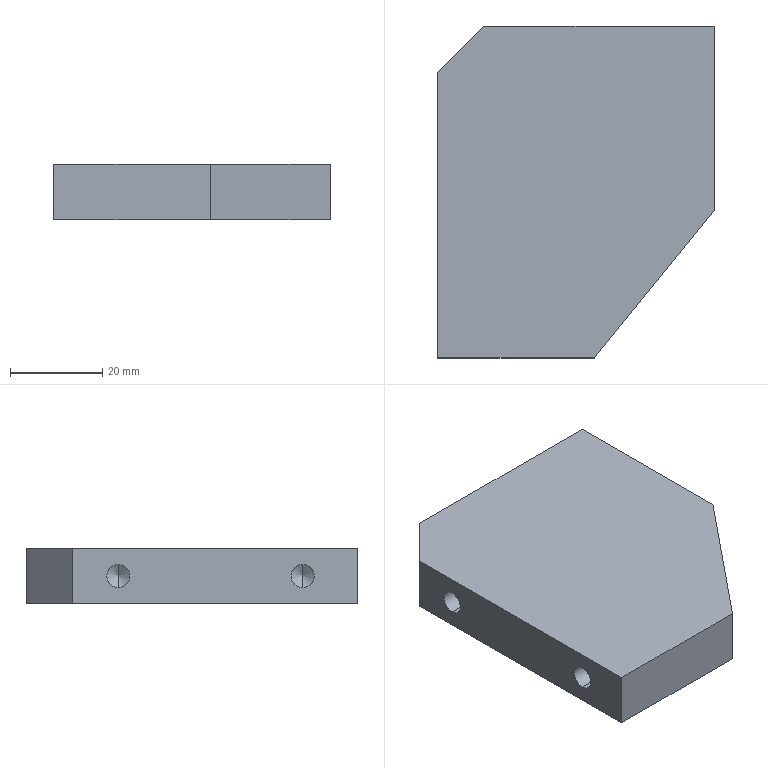Part | SolidWorks | features HoleWzd 2, Chamfer 1, Extrusion 1 | 1 solid | 24 faces | box 60 x 72 x 12 mm | volume 45188 mm3 | cylinder 8 | cone 8 | plane 8 | commonest cylinder face diameters 5 x8
STEP:
#1=CARTESIAN_POINT('',(-86.999,-8.,3.5));
#2=VERTEX_POINT('',#1);
#3=CARTESIAN_POINT('',(-86.999,-8.,8.5));
#4=VERTEX_POINT('',#3);
#5=CARTESIAN_POINT('',(-86.999,-8.,6.));
#6=DIRECTION('',(-1.,0.,0.));
#7=DIRECTION('',(0.,0.,1.));
#8=AXIS2_PLACEMENT_3D('',#5,#6,#7);
#9=CIRCLE('',#8,2.5);
#10=EDGE_CURVE('',#2,#4,#9,.T.);
#11=ORIENTED_EDGE('',*,*,#10,.F.);
#12=CARTESIAN_POINT('',(-99.999,-8.,3.5));
#13=VERTEX_POINT('',#12);
#14=CARTESIAN_POINT('',(-99.999,-8.,3.5));
#15=DIRECTION('',(-1.,0.,0.));
#16=VECTOR('',#15,1000.);
#17=LINE('',#14,#16);
#18=EDGE_CURVE('',#2,#13,#17,.T.);
#19=ORIENTED_EDGE('',*,*,#18,.T.);
#20=CARTESIAN_POINT('',(-99.999,-8.,8.5));
#21=VERTEX_POINT('',#20);
#22=CARTESIAN_POINT('',(-99.999,-8.,6.));
#23=DIRECTION('',(-1.,0.,0.));
#24=DIRECTION('',(0.,0.,1.));
#25=AXIS2_PLACEMENT_3D('',#22,#23,#24);
#26=CIRCLE('',#25,2.5);
#27=EDGE_CURVE('',#13,#21,#26,.T.);
#28=ORIENTED_EDGE('',*,*,#27,.T.);
#29=CARTESIAN_POINT('',(-99.999,-8.,8.5));
#30=DIRECTION('',(-1.,0.,0.));
#31=VECTOR('',#30,1000.);
#32=LINE('',#29,#31);
#33=EDGE_CURVE('',#4,#21,#32,.T.);
#34=ORIENTED_EDGE('',*,*,#33,.F.);
#35=EDGE_LOOP('',(#11,#19,#28,#34));
#36=FACE_OUTER_BOUND('',#35,.T.);
#37=CARTESIAN_POINT('',(-99.999,-8.,6.));
#38=DIRECTION('',(-1.,0.,0.));
#39=DIRECTION('',(0.,0.,1.));
#40=AXIS2_PLACEMENT_3D('',#37,#38,#39);
#41=CYLINDRICAL_SURFACE('',#40,2.5);
#42=ADVANCED_FACE('',(#36),#41,.F.);
#43=CARTESIAN_POINT('',(-85.496,-8.,6.));
#44=VERTEX_POINT('',#43);
#45=CARTESIAN_POINT('',(-86.999,-8.,8.5));
#46=DIRECTION('',(-0.515,0.,0.8572));
#47=VECTOR('',#46,1000.);
#48=LINE('',#45,#47);
#49=EDGE_CURVE('',#44,#4,#48,.T.);
#50=ORIENTED_EDGE('',*,*,#49,.F.);
#51=CARTESIAN_POINT('',(-86.999,-8.,3.5));
#52=DIRECTION('',(-0.515,0.,-0.8572));
#53=VECTOR('',#52,1000.);
#54=LINE('',#51,#53);
#55=EDGE_CURVE('',#44,#2,#54,.T.);
#56=ORIENTED_EDGE('',*,*,#55,.T.);
#57=ORIENTED_EDGE('',*,*,#10,.T.);
#58=EDGE_LOOP('',(#50,#56,#57));
#59=FACE_OUTER_BOUND('',#58,.T.);
#60=CARTESIAN_POINT('',(-86.999,-8.,6.));
#61=DIRECTION('',(-1.,0.,0.));
#62=DIRECTION('',(0.,0.,1.));
#63=AXIS2_PLACEMENT_3D('',#60,#61,#62);
#64=CONICAL_SURFACE('',#63,2.5,1.03);
#65=ADVANCED_FACE('',(#59),#64,.F.);
#66=CARTESIAN_POINT('',(-86.999,-48.,3.5));
#67=VERTEX_POINT('',#66);
#68=CARTESIAN_POINT('',(-86.999,-48.,8.5));
#69=VERTEX_POINT('',#68);
#70=CARTESIAN_POINT('',(-86.999,-48.,6.));
#71=DIRECTION('',(-1.,0.,0.));
#72=DIRECTION('',(0.,0.,1.));
#73=AXIS2_PLACEMENT_3D('',#70,#71,#72);
#74=CIRCLE('',#73,2.5);
#75=EDGE_CURVE('',#67,#69,#74,.T.);
#76=ORIENTED_EDGE('',*,*,#75,.F.);
#77=CARTESIAN_POINT('',(-99.999,-48.,3.5));
#78=VERTEX_POINT('',#77);
#79=CARTESIAN_POINT('',(-99.999,-48.,3.5));
#80=DIRECTION('',(-1.,0.,0.));
#81=VECTOR('',#80,1000.);
#82=LINE('',#79,#81);
#83=EDGE_CURVE('',#67,#78,#82,.T.);
#84=ORIENTED_EDGE('',*,*,#83,.T.);
#85=CARTESIAN_POINT('',(-99.999,-48.,8.5));
#86=VERTEX_POINT('',#85);
#87=CARTESIAN_POINT('',(-99.999,-48.,6.));
#88=DIRECTION('',(-1.,0.,0.));
#89=DIRECTION('',(0.,0.,1.));
#90=AXIS2_PLACEMENT_3D('',#87,#88,#89);
#91=CIRCLE('',#90,2.5);
#92=EDGE_CURVE('',#78,#86,#91,.T.);
#93=ORIENTED_EDGE('',*,*,#92,.T.);
#94=CARTESIAN_POINT('',(-99.999,-48.,8.5));
#95=DIRECTION('',(-1.,0.,0.));
#96=VECTOR('',#95,1000.);
#97=LINE('',#94,#96);
#98=EDGE_CURVE('',#69,#86,#97,.T.);
#99=ORIENTED_EDGE('',*,*,#98,.F.);
#100=EDGE_LOOP('',(#76,#84,#93,#99));
#101=FACE_OUTER_BOUND('',#100,.T.);
#102=CARTESIAN_POINT('',(-99.999,-48.,6.));
#103=DIRECTION('',(-1.,0.,0.));
#104=DIRECTION('',(0.,0.,1.));
#105=AXIS2_PLACEMENT_3D('',#102,#103,#104);
#106=CYLINDRICAL_SURFACE('',#105,2.5);
#107=ADVANCED_FACE('',(#101),#106,.F.);
#108=CARTESIAN_POINT('',(-85.496,-48.,6.));
#109=VERTEX_POINT('',#108);
#110=CARTESIAN_POINT('',(-86.999,-48.,8.5));
#111=DIRECTION('',(-0.515,0.,0.8572));
#112=VECTOR('',#111,1000.);
#113=LINE('',#110,#112);
#114=EDGE_CURVE('',#109,#69,#113,.T.);
#115=ORIENTED_EDGE('',*,*,#114,.F.);
#116=CARTESIAN_POINT('',(-86.999,-48.,3.5));
#117=DIRECTION('',(-0.515,0.,-0.8572));
#118=VECTOR('',#117,1000.);
#119=LINE('',#116,#118);
#120=EDGE_CURVE('',#109,#67,#119,.T.);
#121=ORIENTED_EDGE('',*,*,#120,.T.);
#122=ORIENTED_EDGE('',*,*,#75,.T.);
#123=EDGE_LOOP('',(#115,#121,#122));
#124=FACE_OUTER_BOUND('',#123,.T.);
#125=CARTESIAN_POINT('',(-86.999,-48.,6.));
#126=DIRECTION('',(-1.,0.,0.));
#127=DIRECTION('',(0.,0.,1.));
#128=AXIS2_PLACEMENT_3D('',#125,#126,#127);
#129=CONICAL_SURFACE('',#128,2.5,1.03);
#130=ADVANCED_FACE('',(#124),#129,.F.);
#131=CARTESIAN_POINT('',(-52.999,4.,8.5));
#132=VERTEX_POINT('',#131);
#133=CARTESIAN_POINT('',(-52.999,4.,3.5));
#134=VERTEX_POINT('',#133);
#135=CARTESIAN_POINT('',(-52.999,4.,6.));
#136=DIRECTION('',(1.,0.,0.));
#137=DIRECTION('',(0.,0.,-1.));
#138=AXIS2_PLACEMENT_3D('',#135,#136,#137);
#139=CIRCLE('',#138,2.5);
#140=EDGE_CURVE('',#132,#134,#139,.T.);
#141=ORIENTED_EDGE('',*,*,#140,.F.);
#142=CARTESIAN_POINT('',(-39.999,4.,8.5));
#143=VERTEX_POINT('',#142);
#144=CARTESIAN_POINT('',(-39.999,4.,8.5));
#145=DIRECTION('',(1.,0.,0.));
#146=VECTOR('',#145,1000.);
#147=LINE('',#144,#146);
#148=EDGE_CURVE('',#132,#143,#147,.T.);
#149=ORIENTED_EDGE('',*,*,#148,.T.);
#150=CARTESIAN_POINT('',(-39.999,4.,3.5));
#151=VERTEX_POINT('',#150);
#152=CARTESIAN_POINT('',(-39.999,4.,6.));
#153=DIRECTION('',(1.,0.,0.));
#154=DIRECTION('',(0.,0.,-1.));
#155=AXIS2_PLACEMENT_3D('',#152,#153,#154);
#156=CIRCLE('',#155,2.5);
#157=EDGE_CURVE('',#143,#151,#156,.T.);
#158=ORIENTED_EDGE('',*,*,#157,.T.);
#159=CARTESIAN_POINT('',(-39.999,4.,3.5));
#160=DIRECTION('',(1.,0.,0.));
#161=VECTOR('',#160,1000.);
#162=LINE('',#159,#161);
#163=EDGE_CURVE('',#134,#151,#162,.T.);
#164=ORIENTED_EDGE('',*,*,#163,.F.);
#165=EDGE_LOOP('',(#141,#149,#158,#164));
#166=FACE_OUTER_BOUND('',#165,.T.);
#167=CARTESIAN_POINT('',(-39.999,4.,6.));
#168=DIRECTION('',(1.,0.,0.));
#169=DIRECTION('',(0.,0.,-1.));
#170=AXIS2_PLACEMENT_3D('',#167,#168,#169);
#171=CYLINDRICAL_SURFACE('',#170,2.5);
#172=ADVANCED_FACE('',(#166),#171,.F.);
#173=CARTESIAN_POINT('',(-54.501,4.,6.));
#174=VERTEX_POINT('',#173);
#175=CARTESIAN_POINT('',(-52.999,4.,3.5));
#176=DIRECTION('',(0.515,0.,-0.8572));
#177=VECTOR('',#176,1000.);
#178=LINE('',#175,#177);
#179=EDGE_CURVE('',#174,#134,#178,.T.);
#180=ORIENTED_EDGE('',*,*,#179,.F.);
#181=CARTESIAN_POINT('',(-52.999,4.,8.5));
#182=DIRECTION('',(0.515,0.,0.8572));
#183=VECTOR('',#182,1000.);
#184=LINE('',#181,#183);
#185=EDGE_CURVE('',#174,#132,#184,.T.);
#186=ORIENTED_EDGE('',*,*,#185,.T.);
#187=ORIENTED_EDGE('',*,*,#140,.T.);
#188=EDGE_LOOP('',(#180,#186,#187));
#189=FACE_OUTER_BOUND('',#188,.T.);
#190=CARTESIAN_POINT('',(-52.999,4.,6.));
#191=DIRECTION('',(1.,0.,0.));
#192=DIRECTION('',(0.,0.,-1.));
#193=AXIS2_PLACEMENT_3D('',#190,#191,#192);
#194=CONICAL_SURFACE('',#193,2.5,1.03);
#195=ADVANCED_FACE('',(#189),#194,.F.);
#196=CARTESIAN_POINT('',(-52.999,-16.,8.5));
#197=VERTEX_POINT('',#196);
#198=CARTESIAN_POINT('',(-52.999,-16.,3.5));
#199=VERTEX_POINT('',#198);
#200=CARTESIAN_POINT('',(-52.999,-16.,6.));
#201=DIRECTION('',(1.,0.,0.));
#202=DIRECTION('',(0.,0.,-1.));
#203=AXIS2_PLACEMENT_3D('',#200,#201,#202);
#204=CIRCLE('',#203,2.5);
#205=EDGE_CURVE('',#197,#199,#204,.T.);
#206=ORIENTED_EDGE('',*,*,#205,.F.);
#207=CARTESIAN_POINT('',(-39.999,-16.,8.5));
#208=VERTEX_POINT('',#207);
#209=CARTESIAN_POINT('',(-39.999,-16.,8.5));
#210=DIRECTION('',(1.,0.,0.));
#211=VECTOR('',#210,1000.);
#212=LINE('',#209,#211);
#213=EDGE_CURVE('',#197,#208,#212,.T.);
#214=ORIENTED_EDGE('',*,*,#213,.T.);
#215=CARTESIAN_POINT('',(-39.999,-16.,3.5));
#216=VERTEX_POINT('',#215);
#217=CARTESIAN_POINT('',(-39.999,-16.,6.));
#218=DIRECTION('',(1.,0.,0.));
#219=DIRECTION('',(0.,0.,-1.));
#220=AXIS2_PLACEMENT_3D('',#217,#218,#219);
#221=CIRCLE('',#220,2.5);
#222=EDGE_CURVE('',#208,#216,#221,.T.);
#223=ORIENTED_EDGE('',*,*,#222,.T.);
#224=CARTESIAN_POINT('',(-39.999,-16.,3.5));
#225=DIRECTION('',(1.,0.,0.));
#226=VECTOR('',#225,1000.);
#227=LINE('',#224,#226);
#228=EDGE_CURVE('',#199,#216,#227,.T.);
#229=ORIENTED_EDGE('',*,*,#228,.F.);
#230=EDGE_LOOP('',(#206,#214,#223,#229));
#231=FACE_OUTER_BOUND('',#230,.T.);
#232=CARTESIAN_POINT('',(-39.999,-16.,6.));
#233=DIRECTION('',(1.,0.,0.));
#234=DIRECTION('',(0.,0.,-1.));
#235=AXIS2_PLACEMENT_3D('',#232,#233,#234);
#236=CYLINDRICAL_SURFACE('',#235,2.5);
#237=ADVANCED_FACE('',(#231),#236,.F.);
#238=CARTESIAN_POINT('',(-54.501,-16.,6.));
#239=VERTEX_POINT('',#238);
#240=CARTESIAN_POINT('',(-52.999,-16.,3.5));
#241=DIRECTION('',(0.515,0.,-0.8572));
#242=VECTOR('',#241,1000.);
#243=LINE('',#240,#242);
#244=EDGE_CURVE('',#239,#199,#243,.T.);
#245=ORIENTED_EDGE('',*,*,#244,.F.);
#246=CARTESIAN_POINT('',(-52.999,-16.,8.5));
#247=DIRECTION('',(0.515,0.,0.8572));
#248=VECTOR('',#247,1000.);
#249=LINE('',#246,#248);
#250=EDGE_CURVE('',#239,#197,#249,.T.);
#251=ORIENTED_EDGE('',*,*,#250,.T.);
#252=ORIENTED_EDGE('',*,*,#205,.T.);
#253=EDGE_LOOP('',(#245,#251,#252));
#254=FACE_OUTER_BOUND('',#253,.T.);
#255=CARTESIAN_POINT('',(-52.999,-16.,6.));
#256=DIRECTION('',(1.,0.,0.));
#257=DIRECTION('',(0.,0.,-1.));
#258=AXIS2_PLACEMENT_3D('',#255,#256,#257);
#259=CONICAL_SURFACE('',#258,2.5,1.03);
#260=ADVANCED_FACE('',(#254),#259,.F.);
#261=CARTESIAN_POINT('',(-39.999,12.,0.));
#262=VERTEX_POINT('',#261);
#263=CARTESIAN_POINT('',(-89.999,12.,0.));
#264=VERTEX_POINT('',#263);
#265=CARTESIAN_POINT('',(-99.999,12.,0.));
#266=DIRECTION('',(-1.,0.,0.));
#267=VECTOR('',#266,1000.);
#268=LINE('',#265,#267);
#269=EDGE_CURVE('',#262,#264,#268,.T.);
#270=ORIENTED_EDGE('',*,*,#269,.T.);
#271=CARTESIAN_POINT('',(-89.999,12.,12.));
#272=VERTEX_POINT('',#271);
#273=CARTESIAN_POINT('',(-89.999,12.,12.));
#274=DIRECTION('',(0.,0.,1.));
#275=VECTOR('',#274,1000.);
#276=LINE('',#273,#275);
#277=EDGE_CURVE('',#264,#272,#276,.T.);
#278=ORIENTED_EDGE('',*,*,#277,.T.);
#279=CARTESIAN_POINT('',(-39.999,12.,12.));
#280=VERTEX_POINT('',#279);
#281=CARTESIAN_POINT('',(-99.999,12.,12.));
#282=DIRECTION('',(-1.,0.,0.));
#283=VECTOR('',#282,1000.);
#284=LINE('',#281,#283);
#285=EDGE_CURVE('',#280,#272,#284,.T.);
#286=ORIENTED_EDGE('',*,*,#285,.F.);
#287=CARTESIAN_POINT('',(-39.999,12.,12.));
#288=DIRECTION('',(0.,0.,-1.));
#289=VECTOR('',#288,1000.);
#290=LINE('',#287,#289);
#291=EDGE_CURVE('',#280,#262,#290,.T.);
#292=ORIENTED_EDGE('',*,*,#291,.T.);
#293=EDGE_LOOP('',(#270,#278,#286,#292));
#294=FACE_OUTER_BOUND('',#293,.T.);
#295=CARTESIAN_POINT('',(-99.999,12.,12.));
#296=DIRECTION('',(0.,-1.,0.));
#297=DIRECTION('',(1.,0.,0.));
#298=AXIS2_PLACEMENT_3D('',#295,#296,#297);
#299=PLANE('',#298);
#300=ADVANCED_FACE('',(#294),#299,.F.);
#301=CARTESIAN_POINT('',(-99.999,-8.,6.));
#302=DIRECTION('',(-1.,0.,0.));
#303=DIRECTION('',(0.,0.,1.));
#304=AXIS2_PLACEMENT_3D('',#301,#302,#303);
#305=CIRCLE('',#304,2.5);
#306=EDGE_CURVE('',#21,#13,#305,.T.);
#307=ORIENTED_EDGE('',*,*,#306,.F.);
#308=ORIENTED_EDGE('',*,*,#27,.F.);
#309=EDGE_LOOP('',(#307,#308));
#310=FACE_BOUND('',#309,.T.);
#311=CARTESIAN_POINT('',(-99.999,-48.,6.));
#312=DIRECTION('',(-1.,0.,0.));
#313=DIRECTION('',(0.,0.,1.));
#314=AXIS2_PLACEMENT_3D('',#311,#312,#313);
#315=CIRCLE('',#314,2.5);
#316=EDGE_CURVE('',#86,#78,#315,.T.);
#317=ORIENTED_EDGE('',*,*,#316,.F.);
#318=ORIENTED_EDGE('',*,*,#92,.F.);
#319=EDGE_LOOP('',(#317,#318));
#320=FACE_BOUND('',#319,.T.);
#321=CARTESIAN_POINT('',(-99.999,2.,12.));
#322=VERTEX_POINT('',#321);
#323=CARTESIAN_POINT('',(-99.999,-60.,12.));
#324=VERTEX_POINT('',#323);
#325=CARTESIAN_POINT('',(-99.999,-60.,12.));
#326=DIRECTION('',(0.,-1.,0.));
#327=VECTOR('',#326,1000.);
#328=LINE('',#325,#327);
#329=EDGE_CURVE('',#322,#324,#328,.T.);
#330=ORIENTED_EDGE('',*,*,#329,.F.);
#331=CARTESIAN_POINT('',(-99.999,2.,0.));
#332=VERTEX_POINT('',#331);
#333=CARTESIAN_POINT('',(-99.999,2.,12.));
#334=DIRECTION('',(0.,0.,-1.));
#335=VECTOR('',#334,1000.);
#336=LINE('',#333,#335);
#337=EDGE_CURVE('',#322,#332,#336,.T.);
#338=ORIENTED_EDGE('',*,*,#337,.T.);
#339=CARTESIAN_POINT('',(-99.999,-60.,0.));
#340=VERTEX_POINT('',#339);
#341=CARTESIAN_POINT('',(-99.999,-60.,0.));
#342=DIRECTION('',(0.,-1.,0.));
#343=VECTOR('',#342,1000.);
#344=LINE('',#341,#343);
#345=EDGE_CURVE('',#332,#340,#344,.T.);
#346=ORIENTED_EDGE('',*,*,#345,.T.);
#347=CARTESIAN_POINT('',(-99.999,-60.,12.));
#348=DIRECTION('',(0.,0.,-1.));
#349=VECTOR('',#348,1000.);
#350=LINE('',#347,#349);
#351=EDGE_CURVE('',#324,#340,#350,.T.);
#352=ORIENTED_EDGE('',*,*,#351,.F.);
#353=EDGE_LOOP('',(#330,#338,#346,#352));
#354=FACE_OUTER_BOUND('',#353,.T.);
#355=CARTESIAN_POINT('',(-99.999,-60.,12.));
#356=DIRECTION('',(1.,0.,0.));
#357=DIRECTION('',(0.,0.,-1.));
#358=AXIS2_PLACEMENT_3D('',#355,#356,#357);
#359=PLANE('',#358);
#360=ADVANCED_FACE('',(#310,#320,#354),#359,.F.);
#361=CARTESIAN_POINT('',(-65.999,-60.,0.));
#362=VERTEX_POINT('',#361);
#363=CARTESIAN_POINT('',(-99.999,-60.,0.));
#364=DIRECTION('',(1.,0.,0.));
#365=VECTOR('',#364,1000.);
#366=LINE('',#363,#365);
#367=EDGE_CURVE('',#340,#362,#366,.T.);
#368=ORIENTED_EDGE('',*,*,#367,.T.);
#369=CARTESIAN_POINT('',(-65.999,-60.,12.));
#370=VERTEX_POINT('',#369);
#371=CARTESIAN_POINT('',(-65.999,-60.,12.));
#372=DIRECTION('',(0.,0.,-1.));
#373=VECTOR('',#372,1000.);
#374=LINE('',#371,#373);
#375=EDGE_CURVE('',#370,#362,#374,.T.);
#376=ORIENTED_EDGE('',*,*,#375,.F.);
#377=CARTESIAN_POINT('',(-99.999,-60.,12.));
#378=DIRECTION('',(1.,0.,0.));
#379=VECTOR('',#378,1000.);
#380=LINE('',#377,#379);
#381=EDGE_CURVE('',#324,#370,#380,.T.);
#382=ORIENTED_EDGE('',*,*,#381,.F.);
#383=ORIENTED_EDGE('',*,*,#351,.T.);
#384=EDGE_LOOP('',(#368,#376,#382,#383));
#385=FACE_OUTER_BOUND('',#384,.T.);
#386=CARTESIAN_POINT('',(-99.999,-60.,12.));
#387=DIRECTION('',(0.,1.,0.));
#388=DIRECTION('',(-1.,0.,0.));
#389=AXIS2_PLACEMENT_3D('',#386,#387,#388);
#390=PLANE('',#389);
#391=ADVANCED_FACE('',(#385),#390,.F.);
#392=CARTESIAN_POINT('',(-39.999,-28.,0.));
#393=VERTEX_POINT('',#392);
#394=CARTESIAN_POINT('',(-65.999,-60.,0.));
#395=DIRECTION('',(0.6306,0.7761,0.));
#396=VECTOR('',#395,1000.);
#397=LINE('',#394,#396);
#398=EDGE_CURVE('',#362,#393,#397,.T.);
#399=ORIENTED_EDGE('',*,*,#398,.T.);
#400=CARTESIAN_POINT('',(-39.999,-28.,12.));
#401=VERTEX_POINT('',#400);
#402=CARTESIAN_POINT('',(-39.999,-28.,12.));
#403=DIRECTION('',(0.,0.,-1.));
#404=VECTOR('',#403,1000.);
#405=LINE('',#402,#404);
#406=EDGE_CURVE('',#401,#393,#405,.T.);
#407=ORIENTED_EDGE('',*,*,#406,.F.);
#408=CARTESIAN_POINT('',(-65.999,-60.,12.));
#409=DIRECTION('',(0.6306,0.7761,0.));
#410=VECTOR('',#409,1000.);
#411=LINE('',#408,#410);
#412=EDGE_CURVE('',#370,#401,#411,.T.);
#413=ORIENTED_EDGE('',*,*,#412,.F.);
#414=ORIENTED_EDGE('',*,*,#375,.T.);
#415=EDGE_LOOP('',(#399,#407,#413,#414));
#416=FACE_OUTER_BOUND('',#415,.T.);
#417=CARTESIAN_POINT('',(-65.999,-60.,12.));
#418=DIRECTION('',(-0.7761,0.6306,0.));
#419=DIRECTION('',(-0.6306,-0.7761,0.));
#420=AXIS2_PLACEMENT_3D('',#417,#418,#419);
#421=PLANE('',#420);
#422=ADVANCED_FACE('',(#416),#421,.F.);
#423=CARTESIAN_POINT('',(-39.999,4.,6.));
#424=DIRECTION('',(1.,0.,0.));
#425=DIRECTION('',(0.,0.,-1.));
#426=AXIS2_PLACEMENT_3D('',#423,#424,#425);
#427=CIRCLE('',#426,2.5);
#428=EDGE_CURVE('',#151,#143,#427,.T.);
#429=ORIENTED_EDGE('',*,*,#428,.F.);
#430=ORIENTED_EDGE('',*,*,#157,.F.);
#431=EDGE_LOOP('',(#429,#430));
#432=FACE_BOUND('',#431,.T.);
#433=CARTESIAN_POINT('',(-39.999,-16.,6.));
#434=DIRECTION('',(1.,0.,0.));
#435=DIRECTION('',(0.,0.,-1.));
#436=AXIS2_PLACEMENT_3D('',#433,#434,#435);
#437=CIRCLE('',#436,2.5);
#438=EDGE_CURVE('',#216,#208,#437,.T.);
#439=ORIENTED_EDGE('',*,*,#438,.F.);
#440=ORIENTED_EDGE('',*,*,#222,.F.);
#441=EDGE_LOOP('',(#439,#440));
#442=FACE_BOUND('',#441,.T.);
#443=CARTESIAN_POINT('',(-39.999,12.,0.));
#444=DIRECTION('',(0.,1.,0.));
#445=VECTOR('',#444,1000.);
#446=LINE('',#443,#445);
#447=EDGE_CURVE('',#393,#262,#446,.T.);
#448=ORIENTED_EDGE('',*,*,#447,.T.);
#449=ORIENTED_EDGE('',*,*,#291,.F.);
#450=CARTESIAN_POINT('',(-39.999,12.,12.));
#451=DIRECTION('',(0.,1.,0.));
#452=VECTOR('',#451,1000.);
#453=LINE('',#450,#452);
#454=EDGE_CURVE('',#401,#280,#453,.T.);
#455=ORIENTED_EDGE('',*,*,#454,.F.);
#456=ORIENTED_EDGE('',*,*,#406,.T.);
#457=EDGE_LOOP('',(#448,#449,#455,#456));
#458=FACE_OUTER_BOUND('',#457,.T.);
#459=CARTESIAN_POINT('',(-39.999,12.,12.));
#460=DIRECTION('',(-1.,0.,0.));
#461=DIRECTION('',(0.,-1.,0.));
#462=AXIS2_PLACEMENT_3D('',#459,#460,#461);
#463=PLANE('',#462);
#464=ADVANCED_FACE('',(#432,#442,#458),#463,.F.);
#465=ORIENTED_EDGE('',*,*,#285,.T.);
#466=CARTESIAN_POINT('',(-99.999,2.,12.));
#467=DIRECTION('',(-0.7071,-0.7071,0.));
#468=VECTOR('',#467,1000.);
#469=LINE('',#466,#468);
#470=EDGE_CURVE('',#272,#322,#469,.T.);
#471=ORIENTED_EDGE('',*,*,#470,.T.);
#472=ORIENTED_EDGE('',*,*,#329,.T.);
#473=ORIENTED_EDGE('',*,*,#381,.T.);
#474=ORIENTED_EDGE('',*,*,#412,.T.);
#475=ORIENTED_EDGE('',*,*,#454,.T.);
#476=EDGE_LOOP('',(#465,#471,#472,#473,#474,#475));
#477=FACE_OUTER_BOUND('',#476,.T.);
#478=CARTESIAN_POINT('',(0.,0.,12.));
#479=DIRECTION('',(0.,0.,-1.));
#480=DIRECTION('',(-1.,0.,0.));
#481=AXIS2_PLACEMENT_3D('',#478,#479,#480);
#482=PLANE('',#481);
#483=ADVANCED_FACE('',(#477),#482,.F.);
#484=ORIENTED_EDGE('',*,*,#345,.F.);
#485=CARTESIAN_POINT('',(-50.999,50.999,0.));
#486=DIRECTION('',(0.7071,0.7071,0.));
#487=VECTOR('',#486,1000.);
#488=LINE('',#485,#487);
#489=EDGE_CURVE('',#332,#264,#488,.T.);
#490=ORIENTED_EDGE('',*,*,#489,.T.);
#491=ORIENTED_EDGE('',*,*,#269,.F.);
#492=ORIENTED_EDGE('',*,*,#447,.F.);
#493=ORIENTED_EDGE('',*,*,#398,.F.);
#494=ORIENTED_EDGE('',*,*,#367,.F.);
#495=EDGE_LOOP('',(#484,#490,#491,#492,#493,#494));
#496=FACE_OUTER_BOUND('',#495,.T.);
#497=CARTESIAN_POINT('',(0.,0.,0.));
#498=DIRECTION('',(0.,0.,-1.));
#499=DIRECTION('',(-1.,0.,0.));
#500=AXIS2_PLACEMENT_3D('',#497,#498,#499);
#501=PLANE('',#500);
#502=ADVANCED_FACE('',(#496),#501,.T.);
#503=ORIENTED_EDGE('',*,*,#470,.F.);
#504=ORIENTED_EDGE('',*,*,#277,.F.);
#505=ORIENTED_EDGE('',*,*,#489,.F.);
#506=ORIENTED_EDGE('',*,*,#337,.F.);
#507=EDGE_LOOP('',(#503,#504,#505,#506));
#508=FACE_OUTER_BOUND('',#507,.T.);
#509=CARTESIAN_POINT('',(-99.999,2.,12.));
#510=DIRECTION('',(0.7071,-0.7071,0.));
#511=DIRECTION('',(0.,0.,-1.));
#512=AXIS2_PLACEMENT_3D('',#509,#510,#511);
#513=PLANE('',#512);
#514=ADVANCED_FACE('',(#508),#513,.F.);
#515=ORIENTED_EDGE('',*,*,#250,.F.);
#516=ORIENTED_EDGE('',*,*,#244,.T.);
#517=CARTESIAN_POINT('',(-52.999,-16.,6.));
#518=DIRECTION('',(1.,0.,0.));
#519=DIRECTION('',(0.,0.,-1.));
#520=AXIS2_PLACEMENT_3D('',#517,#518,#519);
#521=CIRCLE('',#520,2.5);
#522=EDGE_CURVE('',#199,#197,#521,.T.);
#523=ORIENTED_EDGE('',*,*,#522,.T.);
#524=EDGE_LOOP('',(#515,#516,#523));
#525=FACE_OUTER_BOUND('',#524,.T.);
#526=CARTESIAN_POINT('',(-52.999,-16.,6.));
#527=DIRECTION('',(1.,0.,0.));
#528=DIRECTION('',(0.,0.,-1.));
#529=AXIS2_PLACEMENT_3D('',#526,#527,#528);
#530=CONICAL_SURFACE('',#529,2.5,1.03);
#531=ADVANCED_FACE('',(#525),#530,.F.);
#532=ORIENTED_EDGE('',*,*,#213,.F.);
#533=ORIENTED_EDGE('',*,*,#522,.F.);
#534=ORIENTED_EDGE('',*,*,#228,.T.);
#535=ORIENTED_EDGE('',*,*,#438,.T.);
#536=EDGE_LOOP('',(#532,#533,#534,#535));
#537=FACE_OUTER_BOUND('',#536,.T.);
#538=CARTESIAN_POINT('',(-39.999,-16.,6.));
#539=DIRECTION('',(1.,0.,0.));
#540=DIRECTION('',(0.,0.,-1.));
#541=AXIS2_PLACEMENT_3D('',#538,#539,#540);
#542=CYLINDRICAL_SURFACE('',#541,2.5);
#543=ADVANCED_FACE('',(#537),#542,.F.);
#544=ORIENTED_EDGE('',*,*,#185,.F.);
#545=ORIENTED_EDGE('',*,*,#179,.T.);
#546=CARTESIAN_POINT('',(-52.999,4.,6.));
#547=DIRECTION('',(1.,0.,0.));
#548=DIRECTION('',(0.,0.,-1.));
#549=AXIS2_PLACEMENT_3D('',#546,#547,#548);
#550=CIRCLE('',#549,2.5);
#551=EDGE_CURVE('',#134,#132,#550,.T.);
#552=ORIENTED_EDGE('',*,*,#551,.T.);
#553=EDGE_LOOP('',(#544,#545,#552));
#554=FACE_OUTER_BOUND('',#553,.T.);
#555=CARTESIAN_POINT('',(-52.999,4.,6.));
#556=DIRECTION('',(1.,0.,0.));
#557=DIRECTION('',(0.,0.,-1.));
#558=AXIS2_PLACEMENT_3D('',#555,#556,#557);
#559=CONICAL_SURFACE('',#558,2.5,1.03);
#560=ADVANCED_FACE('',(#554),#559,.F.);
#561=ORIENTED_EDGE('',*,*,#148,.F.);
#562=ORIENTED_EDGE('',*,*,#551,.F.);
#563=ORIENTED_EDGE('',*,*,#163,.T.);
#564=ORIENTED_EDGE('',*,*,#428,.T.);
#565=EDGE_LOOP('',(#561,#562,#563,#564));
#566=FACE_OUTER_BOUND('',#565,.T.);
#567=CARTESIAN_POINT('',(-39.999,4.,6.));
#568=DIRECTION('',(1.,0.,0.));
#569=DIRECTION('',(0.,0.,-1.));
#570=AXIS2_PLACEMENT_3D('',#567,#568,#569);
#571=CYLINDRICAL_SURFACE('',#570,2.5);
#572=ADVANCED_FACE('',(#566),#571,.F.);
#573=ORIENTED_EDGE('',*,*,#120,.F.);
#574=ORIENTED_EDGE('',*,*,#114,.T.);
#575=CARTESIAN_POINT('',(-86.999,-48.,6.));
#576=DIRECTION('',(-1.,0.,0.));
#577=DIRECTION('',(0.,0.,1.));
#578=AXIS2_PLACEMENT_3D('',#575,#576,#577);
#579=CIRCLE('',#578,2.5);
#580=EDGE_CURVE('',#69,#67,#579,.T.);
#581=ORIENTED_EDGE('',*,*,#580,.T.);
#582=EDGE_LOOP('',(#573,#574,#581));
#583=FACE_OUTER_BOUND('',#582,.T.);
#584=CARTESIAN_POINT('',(-86.999,-48.,6.));
#585=DIRECTION('',(-1.,0.,0.));
#586=DIRECTION('',(0.,0.,1.));
#587=AXIS2_PLACEMENT_3D('',#584,#585,#586);
#588=CONICAL_SURFACE('',#587,2.5,1.03);
#589=ADVANCED_FACE('',(#583),#588,.F.);
#590=ORIENTED_EDGE('',*,*,#83,.F.);
#591=ORIENTED_EDGE('',*,*,#580,.F.);
#592=ORIENTED_EDGE('',*,*,#98,.T.);
#593=ORIENTED_EDGE('',*,*,#316,.T.);
#594=EDGE_LOOP('',(#590,#591,#592,#593));
#595=FACE_OUTER_BOUND('',#594,.T.);
#596=CARTESIAN_POINT('',(-99.999,-48.,6.));
#597=DIRECTION('',(-1.,0.,0.));
#598=DIRECTION('',(0.,0.,1.));
#599=AXIS2_PLACEMENT_3D('',#596,#597,#598);
#600=CYLINDRICAL_SURFACE('',#599,2.5);
#601=ADVANCED_FACE('',(#595),#600,.F.);
#602=ORIENTED_EDGE('',*,*,#55,.F.);
#603=ORIENTED_EDGE('',*,*,#49,.T.);
#604=CARTESIAN_POINT('',(-86.999,-8.,6.));
#605=DIRECTION('',(-1.,0.,0.));
#606=DIRECTION('',(0.,0.,1.));
#607=AXIS2_PLACEMENT_3D('',#604,#605,#606);
#608=CIRCLE('',#607,2.5);
#609=EDGE_CURVE('',#4,#2,#608,.T.);
#610=ORIENTED_EDGE('',*,*,#609,.T.);
#611=EDGE_LOOP('',(#602,#603,#610));
#612=FACE_OUTER_BOUND('',#611,.T.);
#613=CARTESIAN_POINT('',(-86.999,-8.,6.));
#614=DIRECTION('',(-1.,0.,0.));
#615=DIRECTION('',(0.,0.,1.));
#616=AXIS2_PLACEMENT_3D('',#613,#614,#615);
#617=CONICAL_SURFACE('',#616,2.5,1.03);
#618=ADVANCED_FACE('',(#612),#617,.F.);
#619=ORIENTED_EDGE('',*,*,#18,.F.);
#620=ORIENTED_EDGE('',*,*,#609,.F.);
#621=ORIENTED_EDGE('',*,*,#33,.T.);
#622=ORIENTED_EDGE('',*,*,#306,.T.);
#623=EDGE_LOOP('',(#619,#620,#621,#622));
#624=FACE_OUTER_BOUND('',#623,.T.);
#625=CARTESIAN_POINT('',(-99.999,-8.,6.));
#626=DIRECTION('',(-1.,0.,0.));
#627=DIRECTION('',(0.,0.,1.));
#628=AXIS2_PLACEMENT_3D('',#625,#626,#627);
#629=CYLINDRICAL_SURFACE('',#628,2.5);
#630=ADVANCED_FACE('',(#624),#629,.F.);
#631=CLOSED_SHELL('',(#42,#65,#107,#130,#172,#195,#237,#260,#300,#360,#391,#422,#464,#483,#502,#514,#531,#543,#560,#572,#589,#601,#618,#630));
#632=MANIFOLD_SOLID_BREP('',#631);
#633=CARTESIAN_POINT('',(0.,0.,0.));
#634=DIRECTION('',(0.,0.,1.));
#635=DIRECTION('',(1.,0.,0.));
#636=AXIS2_PLACEMENT_3D('',#633,#634,#635);
#637=(LENGTH_UNIT()NAMED_UNIT(*)SI_UNIT(.MILLI.,.METRE.));
#638=UNCERTAINTY_MEASURE_WITH_UNIT(LENGTH_MEASURE(0.00001),#637,'','');
#639=(NAMED_UNIT(*)PLANE_ANGLE_UNIT()SI_UNIT($,.RADIAN.));
#640=(NAMED_UNIT(*)SI_UNIT($,.STERADIAN.)SOLID_ANGLE_UNIT());
#641=(GEOMETRIC_REPRESENTATION_CONTEXT(3)GLOBAL_UNCERTAINTY_ASSIGNED_CONTEXT((#638))GLOBAL_UNIT_ASSIGNED_CONTEXT((#637,#639,#640))REPRESENTATION_CONTEXT('',''));
#642=ADVANCED_BREP_SHAPE_REPRESENTATION('',(#632,#636),#641);